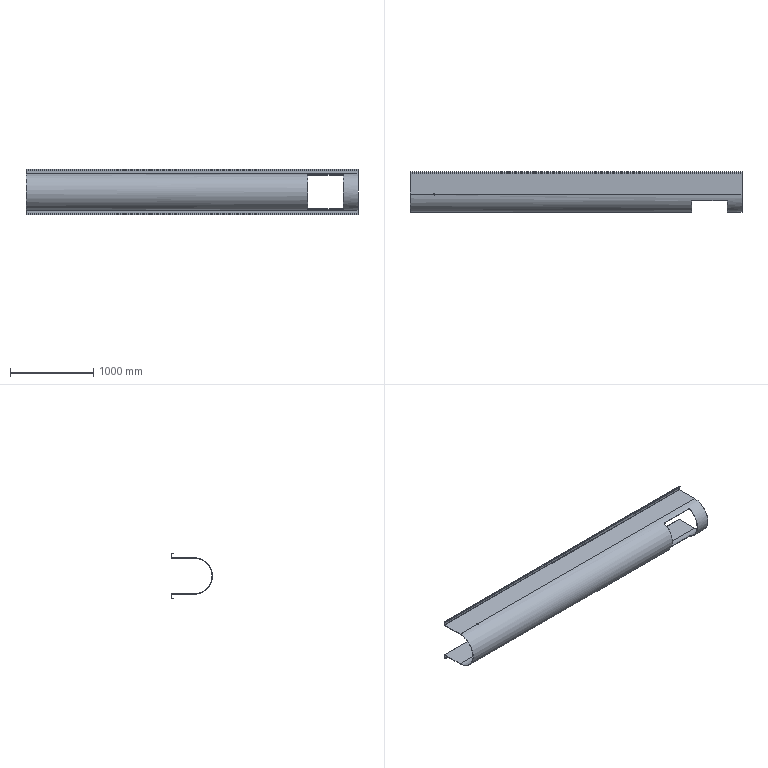Part | STEP file | Input 51 | 1 solid | 54 faces | box 3980 x 490 x 540 mm | volume 25651911 mm3 | plane 40 | cylinder 12 | spline 2 | commonest cylinder face diameters 5 x4 15 x4 20 x2 430 x1 440 x1